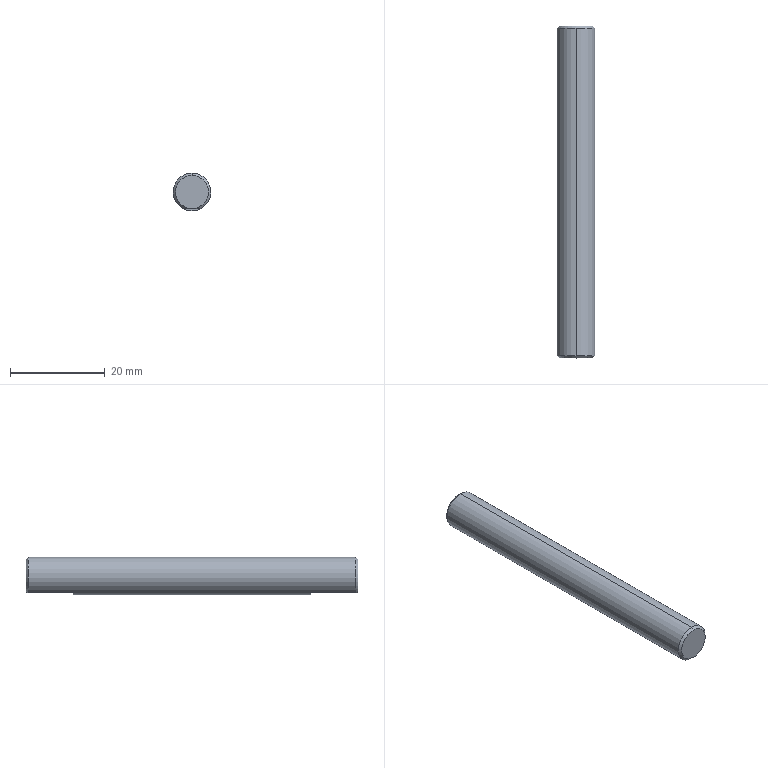Part | SolidWorks | features Chamfer 1, Extrusion 1, ICE 1 | 1 solid | 12 faces | box 8 x 70 x 8 mm | volume 3487 mm3 | plane 6 | cone 4 | cylinder 2 | commonest cylinder face diameters 8 x2
STEP:
#1=CARTESIAN_POINT('',(0.,0.,3.5));
#2=VERTEX_POINT('',#1);
#3=CARTESIAN_POINT('',(0.,0.,-3.5));
#4=VERTEX_POINT('',#3);
#5=CARTESIAN_POINT('',(0.,0.,0.));
#6=DIRECTION('',(0.,-1.,0.));
#7=DIRECTION('',(0.,0.,1.));
#8=AXIS2_PLACEMENT_3D('',#5,#6,#7);
#9=CIRCLE('',#8,3.5);
#10=EDGE_CURVE('',#2,#4,#9,.T.);
#11=ORIENTED_EDGE('',*,*,#10,.F.);
#12=CARTESIAN_POINT('',(0.,0.5,4.));
#13=VERTEX_POINT('',#12);
#14=CARTESIAN_POINT('',(0.,0.5,4.));
#15=DIRECTION('',(0.,0.7071,0.7071));
#16=VECTOR('',#15,1000.);
#17=LINE('',#14,#16);
#18=EDGE_CURVE('',#2,#13,#17,.T.);
#19=ORIENTED_EDGE('',*,*,#18,.T.);
#20=CARTESIAN_POINT('',(-1.936,0.5,-3.5));
#21=VERTEX_POINT('',#20);
#22=CARTESIAN_POINT('',(0.,0.5,0.));
#23=DIRECTION('',(0.,1.,0.));
#24=DIRECTION('',(0.,0.,1.));
#25=AXIS2_PLACEMENT_3D('',#22,#23,#24);
#26=CIRCLE('',#25,4.);
#27=EDGE_CURVE('',#21,#13,#26,.T.);
#28=ORIENTED_EDGE('',*,*,#27,.F.);
#29=CARTESIAN_POINT('',(0.,0.,-3.5));
#30=CARTESIAN_POINT('',(-0.34,0.,-3.5));
#31=CARTESIAN_POINT('',(-0.673,0.05018,-3.5));
#32=CARTESIAN_POINT('',(-1.328,0.2302,-3.5));
#33=CARTESIAN_POINT('',(-1.638,0.3555,-3.5));
#34=CARTESIAN_POINT('',(-1.936,0.5,-3.5));
#35=B_SPLINE_CURVE_WITH_KNOTS('',3,(#29,#30,#31,#32,#33,#34),.UNSPECIFIED.,.F.,.F.,(4,2,4),(0.004182,0.005183,0.006184),.UNSPECIFIED.);
#36=EDGE_CURVE('',#4,#21,#35,.T.);
#37=ORIENTED_EDGE('',*,*,#36,.F.);
#38=EDGE_LOOP('',(#11,#19,#28,#37));
#39=FACE_OUTER_BOUND('',#38,.T.);
#40=CARTESIAN_POINT('',(0.,0.5,0.));
#41=DIRECTION('',(0.,1.,0.));
#42=DIRECTION('',(0.,0.,1.));
#43=AXIS2_PLACEMENT_3D('',#40,#41,#42);
#44=CONICAL_SURFACE('',#43,4.,0.7854);
#45=ADVANCED_FACE('',(#39),#44,.T.);
#46=CARTESIAN_POINT('',(0.,70.,3.5));
#47=VERTEX_POINT('',#46);
#48=CARTESIAN_POINT('',(0.,70.,-3.5));
#49=VERTEX_POINT('',#48);
#50=CARTESIAN_POINT('',(0.,70.,0.));
#51=DIRECTION('',(0.,1.,0.));
#52=DIRECTION('',(0.,0.,1.));
#53=AXIS2_PLACEMENT_3D('',#50,#51,#52);
#54=CIRCLE('',#53,3.5);
#55=EDGE_CURVE('',#47,#49,#54,.T.);
#56=ORIENTED_EDGE('',*,*,#55,.F.);
#57=CARTESIAN_POINT('',(0.,69.5,4.));
#58=VERTEX_POINT('',#57);
#59=CARTESIAN_POINT('',(0.,70.,3.5));
#60=DIRECTION('',(0.,-0.7071,0.7071));
#61=VECTOR('',#60,1000.);
#62=LINE('',#59,#61);
#63=EDGE_CURVE('',#47,#58,#62,.T.);
#64=ORIENTED_EDGE('',*,*,#63,.T.);
#65=CARTESIAN_POINT('',(1.936,69.5,-3.5));
#66=VERTEX_POINT('',#65);
#67=CARTESIAN_POINT('',(0.,69.5,0.));
#68=DIRECTION('',(0.,-1.,0.));
#69=DIRECTION('',(0.,0.,1.));
#70=AXIS2_PLACEMENT_3D('',#67,#68,#69);
#71=CIRCLE('',#70,4.);
#72=EDGE_CURVE('',#66,#58,#71,.T.);
#73=ORIENTED_EDGE('',*,*,#72,.F.);
#74=CARTESIAN_POINT('',(0.,70.,-3.5));
#75=CARTESIAN_POINT('',(0.3393,70.,-3.5));
#76=CARTESIAN_POINT('',(0.6719,69.95,-3.5));
#77=CARTESIAN_POINT('',(1.158,69.817,-3.5));
#78=CARTESIAN_POINT('',(1.319,69.762,-3.5));
#79=CARTESIAN_POINT('',(1.633,69.64,-3.5));
#80=CARTESIAN_POINT('',(1.786,69.573,-3.5));
#81=CARTESIAN_POINT('',(1.936,69.5,-3.5));
#82=B_SPLINE_CURVE_WITH_KNOTS('',3,(#74,#75,#76,#77,#78,#79,#80,#81),.UNSPECIFIED.,.F.,.F.,(4,2,2,4),(0.01206,0.01306,0.01356,0.01406),.UNSPECIFIED.);
#83=EDGE_CURVE('',#49,#66,#82,.T.);
#84=ORIENTED_EDGE('',*,*,#83,.F.);
#85=EDGE_LOOP('',(#56,#64,#73,#84));
#86=FACE_OUTER_BOUND('',#85,.T.);
#87=CARTESIAN_POINT('',(0.,70.,0.));
#88=DIRECTION('',(0.,-1.,0.));
#89=DIRECTION('',(0.,0.,-1.));
#90=AXIS2_PLACEMENT_3D('',#87,#88,#89);
#91=CONICAL_SURFACE('',#90,3.5,0.7854);
#92=ADVANCED_FACE('',(#86),#91,.T.);
#93=ORIENTED_EDGE('',*,*,#72,.T.);
#94=CARTESIAN_POINT('',(0.,70.,4.));
#95=DIRECTION('',(0.,-1.,0.));
#96=VECTOR('',#95,1000.);
#97=LINE('',#94,#96);
#98=EDGE_CURVE('',#58,#13,#97,.T.);
#99=ORIENTED_EDGE('',*,*,#98,.T.);
#100=CARTESIAN_POINT('',(1.936,0.5,-3.5));
#101=VERTEX_POINT('',#100);
#102=CARTESIAN_POINT('',(0.,0.5,0.));
#103=DIRECTION('',(0.,1.,0.));
#104=DIRECTION('',(0.,0.,1.));
#105=AXIS2_PLACEMENT_3D('',#102,#103,#104);
#106=CIRCLE('',#105,4.);
#107=EDGE_CURVE('',#13,#101,#106,.T.);
#108=ORIENTED_EDGE('',*,*,#107,.T.);
#109=CARTESIAN_POINT('',(1.936,10.,-3.5));
#110=VERTEX_POINT('',#109);
#111=CARTESIAN_POINT('',(1.936,70.,-3.5));
#112=DIRECTION('',(0.,1.,0.));
#113=VECTOR('',#112,1000.);
#114=LINE('',#111,#113);
#115=EDGE_CURVE('',#101,#110,#114,.T.);
#116=ORIENTED_EDGE('',*,*,#115,.T.);
#117=CARTESIAN_POINT('',(0.,10.,-4.));
#118=VERTEX_POINT('',#117);
#119=CARTESIAN_POINT('',(0.,10.,0.));
#120=DIRECTION('',(0.,1.,0.));
#121=DIRECTION('',(0.,0.,1.));
#122=AXIS2_PLACEMENT_3D('',#119,#120,#121);
#123=CIRCLE('',#122,4.);
#124=EDGE_CURVE('',#110,#118,#123,.T.);
#125=ORIENTED_EDGE('',*,*,#124,.T.);
#126=CARTESIAN_POINT('',(0.,60.,-4.));
#127=VERTEX_POINT('',#126);
#128=CARTESIAN_POINT('',(0.,70.,-4.));
#129=DIRECTION('',(0.,-1.,0.));
#130=VECTOR('',#129,1000.);
#131=LINE('',#128,#130);
#132=EDGE_CURVE('',#127,#118,#131,.T.);
#133=ORIENTED_EDGE('',*,*,#132,.F.);
#134=CARTESIAN_POINT('',(1.936,60.,-3.5));
#135=VERTEX_POINT('',#134);
#136=CARTESIAN_POINT('',(0.,60.,0.));
#137=DIRECTION('',(0.,-1.,0.));
#138=DIRECTION('',(0.,0.,-1.));
#139=AXIS2_PLACEMENT_3D('',#136,#137,#138);
#140=CIRCLE('',#139,4.);
#141=EDGE_CURVE('',#127,#135,#140,.T.);
#142=ORIENTED_EDGE('',*,*,#141,.T.);
#143=CARTESIAN_POINT('',(1.936,70.,-3.5));
#144=DIRECTION('',(0.,1.,0.));
#145=VECTOR('',#144,1000.);
#146=LINE('',#143,#145);
#147=EDGE_CURVE('',#135,#66,#146,.T.);
#148=ORIENTED_EDGE('',*,*,#147,.T.);
#149=EDGE_LOOP('',(#93,#99,#108,#116,#125,#133,#142,#148));
#150=FACE_OUTER_BOUND('',#149,.T.);
#151=CARTESIAN_POINT('',(0.,70.,0.));
#152=DIRECTION('',(0.,-1.,0.));
#153=DIRECTION('',(0.,0.,-1.));
#154=AXIS2_PLACEMENT_3D('',#151,#152,#153);
#155=CYLINDRICAL_SURFACE('',#154,4.);
#156=ADVANCED_FACE('',(#150),#155,.T.);
#157=ORIENTED_EDGE('',*,*,#98,.F.);
#158=CARTESIAN_POINT('',(-1.936,69.5,-3.5));
#159=VERTEX_POINT('',#158);
#160=CARTESIAN_POINT('',(0.,69.5,0.));
#161=DIRECTION('',(0.,-1.,0.));
#162=DIRECTION('',(0.,0.,1.));
#163=AXIS2_PLACEMENT_3D('',#160,#161,#162);
#164=CIRCLE('',#163,4.);
#165=EDGE_CURVE('',#58,#159,#164,.T.);
#166=ORIENTED_EDGE('',*,*,#165,.T.);
#167=CARTESIAN_POINT('',(-1.936,60.,-3.5));
#168=VERTEX_POINT('',#167);
#169=CARTESIAN_POINT('',(-1.936,70.,-3.5));
#170=DIRECTION('',(0.,-1.,0.));
#171=VECTOR('',#170,1000.);
#172=LINE('',#169,#171);
#173=EDGE_CURVE('',#159,#168,#172,.T.);
#174=ORIENTED_EDGE('',*,*,#173,.T.);
#175=CARTESIAN_POINT('',(0.,60.,0.));
#176=DIRECTION('',(0.,-1.,0.));
#177=DIRECTION('',(0.,0.,-1.));
#178=AXIS2_PLACEMENT_3D('',#175,#176,#177);
#179=CIRCLE('',#178,4.);
#180=EDGE_CURVE('',#168,#127,#179,.T.);
#181=ORIENTED_EDGE('',*,*,#180,.T.);
#182=ORIENTED_EDGE('',*,*,#132,.T.);
#183=CARTESIAN_POINT('',(-1.936,10.,-3.5));
#184=VERTEX_POINT('',#183);
#185=CARTESIAN_POINT('',(0.,10.,0.));
#186=DIRECTION('',(0.,1.,0.));
#187=DIRECTION('',(0.,0.,1.));
#188=AXIS2_PLACEMENT_3D('',#185,#186,#187);
#189=CIRCLE('',#188,4.);
#190=EDGE_CURVE('',#118,#184,#189,.T.);
#191=ORIENTED_EDGE('',*,*,#190,.T.);
#192=CARTESIAN_POINT('',(-1.936,70.,-3.5));
#193=DIRECTION('',(0.,-1.,0.));
#194=VECTOR('',#193,1000.);
#195=LINE('',#192,#194);
#196=EDGE_CURVE('',#184,#21,#195,.T.);
#197=ORIENTED_EDGE('',*,*,#196,.T.);
#198=ORIENTED_EDGE('',*,*,#27,.T.);
#199=EDGE_LOOP('',(#157,#166,#174,#181,#182,#191,#197,#198));
#200=FACE_OUTER_BOUND('',#199,.T.);
#201=CARTESIAN_POINT('',(0.,70.,0.));
#202=DIRECTION('',(0.,-1.,0.));
#203=DIRECTION('',(0.,0.,-1.));
#204=AXIS2_PLACEMENT_3D('',#201,#202,#203);
#205=CYLINDRICAL_SURFACE('',#204,4.);
#206=ADVANCED_FACE('',(#200),#205,.T.);
#207=CARTESIAN_POINT('',(0.,70.,0.));
#208=DIRECTION('',(0.,1.,0.));
#209=DIRECTION('',(0.,0.,1.));
#210=AXIS2_PLACEMENT_3D('',#207,#208,#209);
#211=CIRCLE('',#210,3.5);
#212=EDGE_CURVE('',#49,#47,#211,.T.);
#213=ORIENTED_EDGE('',*,*,#212,.T.);
#214=ORIENTED_EDGE('',*,*,#55,.T.);
#215=EDGE_LOOP('',(#213,#214));
#216=FACE_OUTER_BOUND('',#215,.T.);
#217=CARTESIAN_POINT('',(0.,70.,0.));
#218=DIRECTION('',(0.,1.,0.));
#219=DIRECTION('',(0.,0.,1.));
#220=AXIS2_PLACEMENT_3D('',#217,#218,#219);
#221=PLANE('',#220);
#222=ADVANCED_FACE('',(#216),#221,.T.);
#223=CARTESIAN_POINT('',(0.,0.,0.));
#224=DIRECTION('',(0.,-1.,0.));
#225=DIRECTION('',(0.,0.,1.));
#226=AXIS2_PLACEMENT_3D('',#223,#224,#225);
#227=CIRCLE('',#226,3.5);
#228=EDGE_CURVE('',#4,#2,#227,.T.);
#229=ORIENTED_EDGE('',*,*,#228,.T.);
#230=ORIENTED_EDGE('',*,*,#10,.T.);
#231=EDGE_LOOP('',(#229,#230));
#232=FACE_OUTER_BOUND('',#231,.T.);
#233=CARTESIAN_POINT('',(0.,0.,0.));
#234=DIRECTION('',(0.,1.,0.));
#235=DIRECTION('',(0.,0.,1.));
#236=AXIS2_PLACEMENT_3D('',#233,#234,#235);
#237=PLANE('',#236);
#238=ADVANCED_FACE('',(#232),#237,.F.);
#239=ORIENTED_EDGE('',*,*,#63,.F.);
#240=ORIENTED_EDGE('',*,*,#212,.F.);
#241=CARTESIAN_POINT('',(-1.936,69.5,-3.5));
#242=CARTESIAN_POINT('',(-1.638,69.645,-3.5));
#243=CARTESIAN_POINT('',(-1.328,69.77,-3.5));
#244=CARTESIAN_POINT('',(-0.673,69.95,-3.5));
#245=CARTESIAN_POINT('',(-0.34,70.,-3.5));
#246=CARTESIAN_POINT('',(0.,70.,-3.5));
#247=B_SPLINE_CURVE_WITH_KNOTS('',3,(#241,#242,#243,#244,#245,#246),.UNSPECIFIED.,.F.,.F.,(4,2,4),(0.01007,0.01107,0.01206),.UNSPECIFIED.);
#248=EDGE_CURVE('',#159,#49,#247,.T.);
#249=ORIENTED_EDGE('',*,*,#248,.F.);
#250=ORIENTED_EDGE('',*,*,#165,.F.);
#251=EDGE_LOOP('',(#239,#240,#249,#250));
#252=FACE_OUTER_BOUND('',#251,.T.);
#253=CARTESIAN_POINT('',(0.,70.,0.));
#254=DIRECTION('',(0.,-1.,0.));
#255=DIRECTION('',(0.,0.,-1.));
#256=AXIS2_PLACEMENT_3D('',#253,#254,#255);
#257=CONICAL_SURFACE('',#256,3.5,0.7854);
#258=ADVANCED_FACE('',(#252),#257,.T.);
#259=ORIENTED_EDGE('',*,*,#18,.F.);
#260=ORIENTED_EDGE('',*,*,#228,.F.);
#261=CARTESIAN_POINT('',(1.936,0.5,-3.5));
#262=CARTESIAN_POINT('',(1.786,0.4273,-3.5));
#263=CARTESIAN_POINT('',(1.633,0.3596,-3.5));
#264=CARTESIAN_POINT('',(1.319,0.2376,-3.5));
#265=CARTESIAN_POINT('',(1.158,0.1834,-3.5));
#266=CARTESIAN_POINT('',(0.6719,0.05023,-3.5));
#267=CARTESIAN_POINT('',(0.3393,0.,-3.5));
#268=CARTESIAN_POINT('',(0.,0.,-3.5));
#269=B_SPLINE_CURVE_WITH_KNOTS('',3,(#261,#262,#263,#264,#265,#266,#267,#268),.UNSPECIFIED.,.F.,.F.,(4,2,2,4),(0.002184,0.002684,0.003183,0.004182),.UNSPECIFIED.);
#270=EDGE_CURVE('',#101,#4,#269,.T.);
#271=ORIENTED_EDGE('',*,*,#270,.F.);
#272=ORIENTED_EDGE('',*,*,#107,.F.);
#273=EDGE_LOOP('',(#259,#260,#271,#272));
#274=FACE_OUTER_BOUND('',#273,.T.);
#275=CARTESIAN_POINT('',(0.,0.5,0.));
#276=DIRECTION('',(0.,1.,0.));
#277=DIRECTION('',(0.,0.,1.));
#278=AXIS2_PLACEMENT_3D('',#275,#276,#277);
#279=CONICAL_SURFACE('',#278,4.,0.7854);
#280=ADVANCED_FACE('',(#274),#279,.T.);
#281=CARTESIAN_POINT('',(-5.,60.,-3.5));
#282=DIRECTION('',(1.,0.,0.));
#283=VECTOR('',#282,1000.);
#284=LINE('',#281,#283);
#285=EDGE_CURVE('',#168,#135,#284,.T.);
#286=ORIENTED_EDGE('',*,*,#285,.T.);
#287=ORIENTED_EDGE('',*,*,#141,.F.);
#288=ORIENTED_EDGE('',*,*,#180,.F.);
#289=EDGE_LOOP('',(#286,#287,#288));
#290=FACE_OUTER_BOUND('',#289,.T.);
#291=CARTESIAN_POINT('',(-5.,60.,-3.5));
#292=DIRECTION('',(0.,-1.,0.));
#293=DIRECTION('',(0.,0.,-1.));
#294=AXIS2_PLACEMENT_3D('',#291,#292,#293);
#295=PLANE('',#294);
#296=ADVANCED_FACE('',(#290),#295,.F.);
#297=ORIENTED_EDGE('',*,*,#248,.T.);
#298=ORIENTED_EDGE('',*,*,#83,.T.);
#299=ORIENTED_EDGE('',*,*,#147,.F.);
#300=ORIENTED_EDGE('',*,*,#285,.F.);
#301=ORIENTED_EDGE('',*,*,#173,.F.);
#302=EDGE_LOOP('',(#297,#298,#299,#300,#301));
#303=FACE_OUTER_BOUND('',#302,.T.);
#304=CARTESIAN_POINT('',(-5.,70.,-3.5));
#305=DIRECTION('',(0.,0.,1.));
#306=DIRECTION('',(0.,-1.,0.));
#307=AXIS2_PLACEMENT_3D('',#304,#305,#306);
#308=PLANE('',#307);
#309=ADVANCED_FACE('',(#303),#308,.F.);
#310=CARTESIAN_POINT('',(-5.,10.,-3.5));
#311=DIRECTION('',(1.,0.,0.));
#312=VECTOR('',#311,1000.);
#313=LINE('',#310,#312);
#314=EDGE_CURVE('',#184,#110,#313,.T.);
#315=ORIENTED_EDGE('',*,*,#314,.F.);
#316=ORIENTED_EDGE('',*,*,#190,.F.);
#317=ORIENTED_EDGE('',*,*,#124,.F.);
#318=EDGE_LOOP('',(#315,#316,#317));
#319=FACE_OUTER_BOUND('',#318,.T.);
#320=CARTESIAN_POINT('',(-5.,10.,-3.5));
#321=DIRECTION('',(0.,1.,0.));
#322=DIRECTION('',(0.,0.,1.));
#323=AXIS2_PLACEMENT_3D('',#320,#321,#322);
#324=PLANE('',#323);
#325=ADVANCED_FACE('',(#319),#324,.F.);
#326=ORIENTED_EDGE('',*,*,#314,.T.);
#327=ORIENTED_EDGE('',*,*,#115,.F.);
#328=ORIENTED_EDGE('',*,*,#270,.T.);
#329=ORIENTED_EDGE('',*,*,#36,.T.);
#330=ORIENTED_EDGE('',*,*,#196,.F.);
#331=EDGE_LOOP('',(#326,#327,#328,#329,#330));
#332=FACE_OUTER_BOUND('',#331,.T.);
#333=CARTESIAN_POINT('',(-5.,0.,-3.5));
#334=DIRECTION('',(0.,0.,1.));
#335=DIRECTION('',(0.,-1.,0.));
#336=AXIS2_PLACEMENT_3D('',#333,#334,#335);
#337=PLANE('',#336);
#338=ADVANCED_FACE('',(#332),#337,.F.);
#339=CLOSED_SHELL('',(#45,#92,#156,#206,#222,#238,#258,#280,#296,#309,#325,#338));
#340=MANIFOLD_SOLID_BREP('',#339);
#341=CARTESIAN_POINT('',(0.,0.,0.));
#342=DIRECTION('',(0.,0.,1.));
#343=DIRECTION('',(1.,0.,0.));
#344=AXIS2_PLACEMENT_3D('',#341,#342,#343);
#345=(LENGTH_UNIT()NAMED_UNIT(*)SI_UNIT(.MILLI.,.METRE.));
#346=UNCERTAINTY_MEASURE_WITH_UNIT(LENGTH_MEASURE(0.00001),#345,'','');
#347=(NAMED_UNIT(*)PLANE_ANGLE_UNIT()SI_UNIT($,.RADIAN.));
#348=(NAMED_UNIT(*)SI_UNIT($,.STERADIAN.)SOLID_ANGLE_UNIT());
#349=(GEOMETRIC_REPRESENTATION_CONTEXT(3)GLOBAL_UNCERTAINTY_ASSIGNED_CONTEXT((#346))GLOBAL_UNIT_ASSIGNED_CONTEXT((#345,#347,#348))REPRESENTATION_CONTEXT('',''));
#350=ADVANCED_BREP_SHAPE_REPRESENTATION('',(#340,#344),#349);